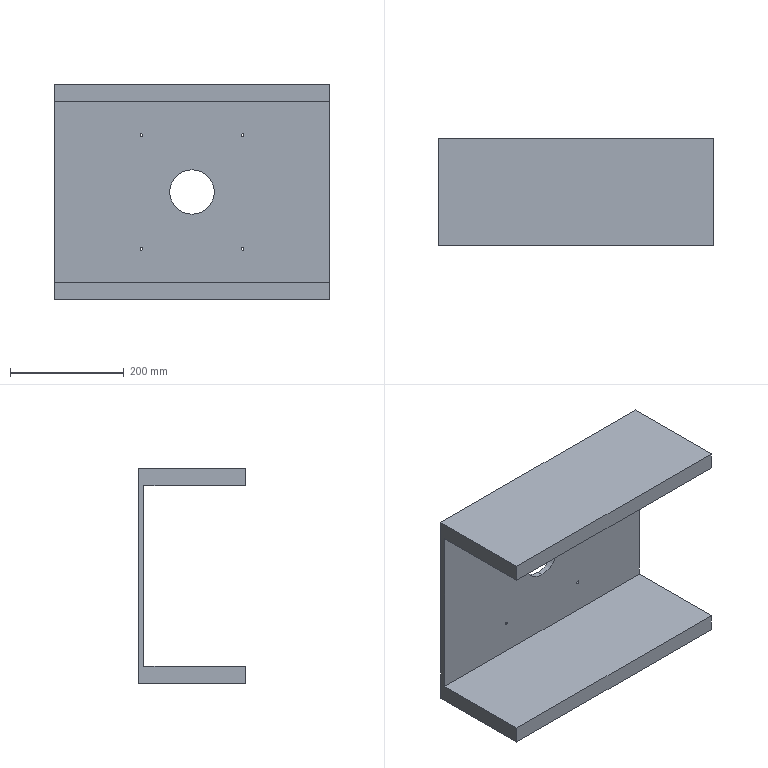Part | SolidWorks | features ICE 2, Extrusion 1 | 1 solid | 20 faces | box 484 x 189 x 378 mm | volume 6979121 mm3 | cylinder 10 | plane 10 | commonest cylinder face diameters 4.5 x8 78.113 x2
STEP:
#1=CARTESIAN_POINT('',(89.,179.,97.75));
#2=VERTEX_POINT('',#1);
#3=CARTESIAN_POINT('',(89.,179.,102.25));
#4=VERTEX_POINT('',#3);
#5=CARTESIAN_POINT('',(89.,179.,100.));
#6=DIRECTION('',(0.,1.,0.));
#7=DIRECTION('',(0.,0.,1.));
#8=AXIS2_PLACEMENT_3D('',#5,#6,#7);
#9=CIRCLE('',#8,2.25);
#10=EDGE_CURVE('',#2,#4,#9,.T.);
#11=ORIENTED_EDGE('',*,*,#10,.F.);
#12=CARTESIAN_POINT('',(89.,189.,97.75));
#13=VERTEX_POINT('',#12);
#14=CARTESIAN_POINT('',(89.,0.,97.75));
#15=DIRECTION('',(0.,1.,0.));
#16=VECTOR('',#15,1000.);
#17=LINE('',#14,#16);
#18=EDGE_CURVE('',#2,#13,#17,.T.);
#19=ORIENTED_EDGE('',*,*,#18,.T.);
#20=CARTESIAN_POINT('',(89.,189.,102.25));
#21=VERTEX_POINT('',#20);
#22=CARTESIAN_POINT('',(89.,189.,100.));
#23=DIRECTION('',(0.,1.,0.));
#24=DIRECTION('',(0.,0.,1.));
#25=AXIS2_PLACEMENT_3D('',#22,#23,#24);
#26=CIRCLE('',#25,2.25);
#27=EDGE_CURVE('',#13,#21,#26,.T.);
#28=ORIENTED_EDGE('',*,*,#27,.T.);
#29=CARTESIAN_POINT('',(89.,0.,102.25));
#30=DIRECTION('',(0.,1.,0.));
#31=VECTOR('',#30,1000.);
#32=LINE('',#29,#31);
#33=EDGE_CURVE('',#4,#21,#32,.T.);
#34=ORIENTED_EDGE('',*,*,#33,.F.);
#35=EDGE_LOOP('',(#11,#19,#28,#34));
#36=FACE_OUTER_BOUND('',#35,.T.);
#37=CARTESIAN_POINT('',(89.,0.,100.));
#38=DIRECTION('',(0.,1.,0.));
#39=DIRECTION('',(0.,0.,1.));
#40=AXIS2_PLACEMENT_3D('',#37,#38,#39);
#41=CYLINDRICAL_SURFACE('',#40,2.25);
#42=ADVANCED_FACE('',(#36),#41,.F.);
#43=CARTESIAN_POINT('',(-89.,179.,-102.25));
#44=VERTEX_POINT('',#43);
#45=CARTESIAN_POINT('',(-89.,179.,-97.75));
#46=VERTEX_POINT('',#45);
#47=CARTESIAN_POINT('',(-89.,179.,-100.));
#48=DIRECTION('',(0.,1.,0.));
#49=DIRECTION('',(0.,0.,1.));
#50=AXIS2_PLACEMENT_3D('',#47,#48,#49);
#51=CIRCLE('',#50,2.25);
#52=EDGE_CURVE('',#44,#46,#51,.T.);
#53=ORIENTED_EDGE('',*,*,#52,.F.);
#54=CARTESIAN_POINT('',(-89.,189.,-102.25));
#55=VERTEX_POINT('',#54);
#56=CARTESIAN_POINT('',(-89.,0.,-102.25));
#57=DIRECTION('',(0.,1.,0.));
#58=VECTOR('',#57,1000.);
#59=LINE('',#56,#58);
#60=EDGE_CURVE('',#44,#55,#59,.T.);
#61=ORIENTED_EDGE('',*,*,#60,.T.);
#62=CARTESIAN_POINT('',(-89.,189.,-97.75));
#63=VERTEX_POINT('',#62);
#64=CARTESIAN_POINT('',(-89.,189.,-100.));
#65=DIRECTION('',(0.,1.,0.));
#66=DIRECTION('',(0.,0.,1.));
#67=AXIS2_PLACEMENT_3D('',#64,#65,#66);
#68=CIRCLE('',#67,2.25);
#69=EDGE_CURVE('',#55,#63,#68,.T.);
#70=ORIENTED_EDGE('',*,*,#69,.T.);
#71=CARTESIAN_POINT('',(-89.,0.,-97.75));
#72=DIRECTION('',(0.,1.,0.));
#73=VECTOR('',#72,1000.);
#74=LINE('',#71,#73);
#75=EDGE_CURVE('',#46,#63,#74,.T.);
#76=ORIENTED_EDGE('',*,*,#75,.F.);
#77=EDGE_LOOP('',(#53,#61,#70,#76));
#78=FACE_OUTER_BOUND('',#77,.T.);
#79=CARTESIAN_POINT('',(-89.,0.,-100.));
#80=DIRECTION('',(0.,1.,0.));
#81=DIRECTION('',(0.,0.,1.));
#82=AXIS2_PLACEMENT_3D('',#79,#80,#81);
#83=CYLINDRICAL_SURFACE('',#82,2.25);
#84=ADVANCED_FACE('',(#78),#83,.F.);
#85=CARTESIAN_POINT('',(89.,179.,-102.25));
#86=VERTEX_POINT('',#85);
#87=CARTESIAN_POINT('',(89.,179.,-97.75));
#88=VERTEX_POINT('',#87);
#89=CARTESIAN_POINT('',(89.,179.,-100.));
#90=DIRECTION('',(0.,1.,0.));
#91=DIRECTION('',(0.,0.,1.));
#92=AXIS2_PLACEMENT_3D('',#89,#90,#91);
#93=CIRCLE('',#92,2.25);
#94=EDGE_CURVE('',#86,#88,#93,.T.);
#95=ORIENTED_EDGE('',*,*,#94,.F.);
#96=CARTESIAN_POINT('',(89.,189.,-102.25));
#97=VERTEX_POINT('',#96);
#98=CARTESIAN_POINT('',(89.,0.,-102.25));
#99=DIRECTION('',(0.,1.,0.));
#100=VECTOR('',#99,1000.);
#101=LINE('',#98,#100);
#102=EDGE_CURVE('',#86,#97,#101,.T.);
#103=ORIENTED_EDGE('',*,*,#102,.T.);
#104=CARTESIAN_POINT('',(89.,189.,-97.75));
#105=VERTEX_POINT('',#104);
#106=CARTESIAN_POINT('',(89.,189.,-100.));
#107=DIRECTION('',(0.,1.,0.));
#108=DIRECTION('',(0.,0.,1.));
#109=AXIS2_PLACEMENT_3D('',#106,#107,#108);
#110=CIRCLE('',#109,2.25);
#111=EDGE_CURVE('',#97,#105,#110,.T.);
#112=ORIENTED_EDGE('',*,*,#111,.T.);
#113=CARTESIAN_POINT('',(89.,0.,-97.75));
#114=DIRECTION('',(0.,1.,0.));
#115=VECTOR('',#114,1000.);
#116=LINE('',#113,#115);
#117=EDGE_CURVE('',#88,#105,#116,.T.);
#118=ORIENTED_EDGE('',*,*,#117,.F.);
#119=EDGE_LOOP('',(#95,#103,#112,#118));
#120=FACE_OUTER_BOUND('',#119,.T.);
#121=CARTESIAN_POINT('',(89.,0.,-100.));
#122=DIRECTION('',(0.,1.,0.));
#123=DIRECTION('',(0.,0.,1.));
#124=AXIS2_PLACEMENT_3D('',#121,#122,#123);
#125=CYLINDRICAL_SURFACE('',#124,2.25);
#126=ADVANCED_FACE('',(#120),#125,.F.);
#127=CARTESIAN_POINT('',(0.,179.,-39.057));
#128=VERTEX_POINT('',#127);
#129=CARTESIAN_POINT('',(0.,179.,39.057));
#130=VERTEX_POINT('',#129);
#131=CARTESIAN_POINT('',(0.,179.,0.));
#132=DIRECTION('',(0.,1.,0.));
#133=DIRECTION('',(0.,0.,1.));
#134=AXIS2_PLACEMENT_3D('',#131,#132,#133);
#135=CIRCLE('',#134,39.057);
#136=EDGE_CURVE('',#128,#130,#135,.T.);
#137=ORIENTED_EDGE('',*,*,#136,.F.);
#138=CARTESIAN_POINT('',(0.,189.,-39.057));
#139=VERTEX_POINT('',#138);
#140=CARTESIAN_POINT('',(0.,0.,-39.057));
#141=DIRECTION('',(0.,1.,0.));
#142=VECTOR('',#141,1000.);
#143=LINE('',#140,#142);
#144=EDGE_CURVE('',#128,#139,#143,.T.);
#145=ORIENTED_EDGE('',*,*,#144,.T.);
#146=CARTESIAN_POINT('',(0.,189.,39.057));
#147=VERTEX_POINT('',#146);
#148=CARTESIAN_POINT('',(0.,189.,0.));
#149=DIRECTION('',(0.,1.,0.));
#150=DIRECTION('',(0.,0.,1.));
#151=AXIS2_PLACEMENT_3D('',#148,#149,#150);
#152=CIRCLE('',#151,39.057);
#153=EDGE_CURVE('',#139,#147,#152,.T.);
#154=ORIENTED_EDGE('',*,*,#153,.T.);
#155=CARTESIAN_POINT('',(0.,0.,39.057));
#156=DIRECTION('',(0.,1.,0.));
#157=VECTOR('',#156,1000.);
#158=LINE('',#155,#157);
#159=EDGE_CURVE('',#130,#147,#158,.T.);
#160=ORIENTED_EDGE('',*,*,#159,.F.);
#161=EDGE_LOOP('',(#137,#145,#154,#160));
#162=FACE_OUTER_BOUND('',#161,.T.);
#163=CARTESIAN_POINT('',(0.,0.,0.));
#164=DIRECTION('',(0.,1.,0.));
#165=DIRECTION('',(0.,0.,1.));
#166=AXIS2_PLACEMENT_3D('',#163,#164,#165);
#167=CYLINDRICAL_SURFACE('',#166,39.057);
#168=ADVANCED_FACE('',(#162),#167,.F.);
#169=CARTESIAN_POINT('',(-89.,179.,97.75));
#170=VERTEX_POINT('',#169);
#171=CARTESIAN_POINT('',(-89.,179.,102.25));
#172=VERTEX_POINT('',#171);
#173=CARTESIAN_POINT('',(-89.,179.,100.));
#174=DIRECTION('',(0.,1.,0.));
#175=DIRECTION('',(0.,0.,1.));
#176=AXIS2_PLACEMENT_3D('',#173,#174,#175);
#177=CIRCLE('',#176,2.25);
#178=EDGE_CURVE('',#170,#172,#177,.T.);
#179=ORIENTED_EDGE('',*,*,#178,.F.);
#180=CARTESIAN_POINT('',(-89.,189.,97.75));
#181=VERTEX_POINT('',#180);
#182=CARTESIAN_POINT('',(-89.,0.,97.75));
#183=DIRECTION('',(0.,1.,0.));
#184=VECTOR('',#183,1000.);
#185=LINE('',#182,#184);
#186=EDGE_CURVE('',#170,#181,#185,.T.);
#187=ORIENTED_EDGE('',*,*,#186,.T.);
#188=CARTESIAN_POINT('',(-89.,189.,102.25));
#189=VERTEX_POINT('',#188);
#190=CARTESIAN_POINT('',(-89.,189.,100.));
#191=DIRECTION('',(0.,1.,0.));
#192=DIRECTION('',(0.,0.,1.));
#193=AXIS2_PLACEMENT_3D('',#190,#191,#192);
#194=CIRCLE('',#193,2.25);
#195=EDGE_CURVE('',#181,#189,#194,.T.);
#196=ORIENTED_EDGE('',*,*,#195,.T.);
#197=CARTESIAN_POINT('',(-89.,0.,102.25));
#198=DIRECTION('',(0.,1.,0.));
#199=VECTOR('',#198,1000.);
#200=LINE('',#197,#199);
#201=EDGE_CURVE('',#172,#189,#200,.T.);
#202=ORIENTED_EDGE('',*,*,#201,.F.);
#203=EDGE_LOOP('',(#179,#187,#196,#202));
#204=FACE_OUTER_BOUND('',#203,.T.);
#205=CARTESIAN_POINT('',(-89.,0.,100.));
#206=DIRECTION('',(0.,1.,0.));
#207=DIRECTION('',(0.,0.,1.));
#208=AXIS2_PLACEMENT_3D('',#205,#206,#207);
#209=CYLINDRICAL_SURFACE('',#208,2.25);
#210=ADVANCED_FACE('',(#204),#209,.F.);
#211=CARTESIAN_POINT('',(242.,0.,-159.));
#212=VERTEX_POINT('',#211);
#213=CARTESIAN_POINT('',(-242.,0.,-159.));
#214=VERTEX_POINT('',#213);
#215=CARTESIAN_POINT('',(242.,0.,-159.));
#216=DIRECTION('',(-1.,0.,0.));
#217=VECTOR('',#216,1000.);
#218=LINE('',#215,#217);
#219=EDGE_CURVE('',#212,#214,#218,.T.);
#220=ORIENTED_EDGE('',*,*,#219,.T.);
#221=CARTESIAN_POINT('',(-242.,0.,-189.));
#222=VERTEX_POINT('',#221);
#223=CARTESIAN_POINT('',(-242.,0.,189.));
#224=DIRECTION('',(0.,0.,1.));
#225=VECTOR('',#224,1000.);
#226=LINE('',#223,#225);
#227=EDGE_CURVE('',#222,#214,#226,.T.);
#228=ORIENTED_EDGE('',*,*,#227,.F.);
#229=CARTESIAN_POINT('',(242.,0.,-189.));
#230=VERTEX_POINT('',#229);
#231=CARTESIAN_POINT('',(-242.,0.,-189.));
#232=DIRECTION('',(-1.,0.,0.));
#233=VECTOR('',#232,1000.);
#234=LINE('',#231,#233);
#235=EDGE_CURVE('',#230,#222,#234,.T.);
#236=ORIENTED_EDGE('',*,*,#235,.F.);
#237=CARTESIAN_POINT('',(242.,0.,189.));
#238=DIRECTION('',(0.,0.,-1.));
#239=VECTOR('',#238,1000.);
#240=LINE('',#237,#239);
#241=EDGE_CURVE('',#212,#230,#240,.T.);
#242=ORIENTED_EDGE('',*,*,#241,.F.);
#243=EDGE_LOOP('',(#220,#228,#236,#242));
#244=FACE_OUTER_BOUND('',#243,.T.);
#245=CARTESIAN_POINT('',(0.,0.,0.));
#246=DIRECTION('',(0.,-1.,0.));
#247=DIRECTION('',(0.,0.,-1.));
#248=AXIS2_PLACEMENT_3D('',#245,#246,#247);
#249=PLANE('',#248);
#250=ADVANCED_FACE('',(#244),#249,.T.);
#251=CARTESIAN_POINT('',(242.,179.,159.));
#252=VERTEX_POINT('',#251);
#253=CARTESIAN_POINT('',(242.,179.,-159.));
#254=VERTEX_POINT('',#253);
#255=CARTESIAN_POINT('',(242.,179.,-159.));
#256=DIRECTION('',(0.,0.,-1.));
#257=VECTOR('',#256,1000.);
#258=LINE('',#255,#257);
#259=EDGE_CURVE('',#252,#254,#258,.T.);
#260=ORIENTED_EDGE('',*,*,#259,.T.);
#261=CARTESIAN_POINT('',(242.,0.,-159.));
#262=DIRECTION('',(0.,-1.,0.));
#263=VECTOR('',#262,1000.);
#264=LINE('',#261,#263);
#265=EDGE_CURVE('',#254,#212,#264,.T.);
#266=ORIENTED_EDGE('',*,*,#265,.T.);
#267=ORIENTED_EDGE('',*,*,#241,.T.);
#268=CARTESIAN_POINT('',(242.,189.,-189.));
#269=VERTEX_POINT('',#268);
#270=CARTESIAN_POINT('',(242.,189.,-189.));
#271=DIRECTION('',(0.,-1.,0.));
#272=VECTOR('',#271,1000.);
#273=LINE('',#270,#272);
#274=EDGE_CURVE('',#269,#230,#273,.T.);
#275=ORIENTED_EDGE('',*,*,#274,.F.);
#276=CARTESIAN_POINT('',(242.,189.,189.));
#277=VERTEX_POINT('',#276);
#278=CARTESIAN_POINT('',(242.,189.,189.));
#279=DIRECTION('',(0.,0.,-1.));
#280=VECTOR('',#279,1000.);
#281=LINE('',#278,#280);
#282=EDGE_CURVE('',#277,#269,#281,.T.);
#283=ORIENTED_EDGE('',*,*,#282,.F.);
#284=CARTESIAN_POINT('',(242.,0.,189.));
#285=VERTEX_POINT('',#284);
#286=CARTESIAN_POINT('',(242.,189.,189.));
#287=DIRECTION('',(0.,-1.,0.));
#288=VECTOR('',#287,1000.);
#289=LINE('',#286,#288);
#290=EDGE_CURVE('',#277,#285,#289,.T.);
#291=ORIENTED_EDGE('',*,*,#290,.T.);
#292=CARTESIAN_POINT('',(242.,0.,159.));
#293=VERTEX_POINT('',#292);
#294=CARTESIAN_POINT('',(242.,0.,189.));
#295=DIRECTION('',(0.,0.,-1.));
#296=VECTOR('',#295,1000.);
#297=LINE('',#294,#296);
#298=EDGE_CURVE('',#285,#293,#297,.T.);
#299=ORIENTED_EDGE('',*,*,#298,.T.);
#300=CARTESIAN_POINT('',(242.,0.,159.));
#301=DIRECTION('',(0.,1.,0.));
#302=VECTOR('',#301,1000.);
#303=LINE('',#300,#302);
#304=EDGE_CURVE('',#293,#252,#303,.T.);
#305=ORIENTED_EDGE('',*,*,#304,.T.);
#306=EDGE_LOOP('',(#260,#266,#267,#275,#283,#291,#299,#305));
#307=FACE_OUTER_BOUND('',#306,.T.);
#308=CARTESIAN_POINT('',(242.,189.,189.));
#309=DIRECTION('',(-1.,0.,0.));
#310=DIRECTION('',(0.,0.,1.));
#311=AXIS2_PLACEMENT_3D('',#308,#309,#310);
#312=PLANE('',#311);
#313=ADVANCED_FACE('',(#307),#312,.F.);
#314=ORIENTED_EDGE('',*,*,#235,.T.);
#315=CARTESIAN_POINT('',(-242.,189.,-189.));
#316=VERTEX_POINT('',#315);
#317=CARTESIAN_POINT('',(-242.,189.,-189.));
#318=DIRECTION('',(0.,-1.,0.));
#319=VECTOR('',#318,1000.);
#320=LINE('',#317,#319);
#321=EDGE_CURVE('',#316,#222,#320,.T.);
#322=ORIENTED_EDGE('',*,*,#321,.F.);
#323=CARTESIAN_POINT('',(-242.,189.,-189.));
#324=DIRECTION('',(-1.,0.,0.));
#325=VECTOR('',#324,1000.);
#326=LINE('',#323,#325);
#327=EDGE_CURVE('',#269,#316,#326,.T.);
#328=ORIENTED_EDGE('',*,*,#327,.F.);
#329=ORIENTED_EDGE('',*,*,#274,.T.);
#330=EDGE_LOOP('',(#314,#322,#328,#329));
#331=FACE_OUTER_BOUND('',#330,.T.);
#332=CARTESIAN_POINT('',(-242.,189.,-189.));
#333=DIRECTION('',(0.,0.,1.));
#334=DIRECTION('',(1.,0.,0.));
#335=AXIS2_PLACEMENT_3D('',#332,#333,#334);
#336=PLANE('',#335);
#337=ADVANCED_FACE('',(#331),#336,.F.);
#338=ORIENTED_EDGE('',*,*,#227,.T.);
#339=CARTESIAN_POINT('',(-242.,179.,-159.));
#340=VERTEX_POINT('',#339);
#341=CARTESIAN_POINT('',(-242.,0.,-159.));
#342=DIRECTION('',(0.,-1.,0.));
#343=VECTOR('',#342,1000.);
#344=LINE('',#341,#343);
#345=EDGE_CURVE('',#340,#214,#344,.T.);
#346=ORIENTED_EDGE('',*,*,#345,.F.);
#347=CARTESIAN_POINT('',(-242.,179.,159.));
#348=VERTEX_POINT('',#347);
#349=CARTESIAN_POINT('',(-242.,179.,-159.));
#350=DIRECTION('',(0.,0.,-1.));
#351=VECTOR('',#350,1000.);
#352=LINE('',#349,#351);
#353=EDGE_CURVE('',#348,#340,#352,.T.);
#354=ORIENTED_EDGE('',*,*,#353,.F.);
#355=CARTESIAN_POINT('',(-242.,0.,159.));
#356=VERTEX_POINT('',#355);
#357=CARTESIAN_POINT('',(-242.,0.,159.));
#358=DIRECTION('',(0.,1.,0.));
#359=VECTOR('',#358,1000.);
#360=LINE('',#357,#359);
#361=EDGE_CURVE('',#356,#348,#360,.T.);
#362=ORIENTED_EDGE('',*,*,#361,.F.);
#363=CARTESIAN_POINT('',(-242.,0.,189.));
#364=VERTEX_POINT('',#363);
#365=CARTESIAN_POINT('',(-242.,0.,189.));
#366=DIRECTION('',(0.,0.,1.));
#367=VECTOR('',#366,1000.);
#368=LINE('',#365,#367);
#369=EDGE_CURVE('',#356,#364,#368,.T.);
#370=ORIENTED_EDGE('',*,*,#369,.T.);
#371=CARTESIAN_POINT('',(-242.,189.,189.));
#372=VERTEX_POINT('',#371);
#373=CARTESIAN_POINT('',(-242.,189.,189.));
#374=DIRECTION('',(0.,-1.,0.));
#375=VECTOR('',#374,1000.);
#376=LINE('',#373,#375);
#377=EDGE_CURVE('',#372,#364,#376,.T.);
#378=ORIENTED_EDGE('',*,*,#377,.F.);
#379=CARTESIAN_POINT('',(-242.,189.,189.));
#380=DIRECTION('',(0.,0.,1.));
#381=VECTOR('',#380,1000.);
#382=LINE('',#379,#381);
#383=EDGE_CURVE('',#316,#372,#382,.T.);
#384=ORIENTED_EDGE('',*,*,#383,.F.);
#385=ORIENTED_EDGE('',*,*,#321,.T.);
#386=EDGE_LOOP('',(#338,#346,#354,#362,#370,#378,#384,#385));
#387=FACE_OUTER_BOUND('',#386,.T.);
#388=CARTESIAN_POINT('',(-242.,189.,189.));
#389=DIRECTION('',(1.,0.,0.));
#390=DIRECTION('',(0.,0.,-1.));
#391=AXIS2_PLACEMENT_3D('',#388,#389,#390);
#392=PLANE('',#391);
#393=ADVANCED_FACE('',(#387),#392,.F.);
#394=CARTESIAN_POINT('',(-242.,0.,189.));
#395=DIRECTION('',(1.,0.,0.));
#396=VECTOR('',#395,1000.);
#397=LINE('',#394,#396);
#398=EDGE_CURVE('',#364,#285,#397,.T.);
#399=ORIENTED_EDGE('',*,*,#398,.T.);
#400=ORIENTED_EDGE('',*,*,#290,.F.);
#401=CARTESIAN_POINT('',(-242.,189.,189.));
#402=DIRECTION('',(1.,0.,0.));
#403=VECTOR('',#402,1000.);
#404=LINE('',#401,#403);
#405=EDGE_CURVE('',#372,#277,#404,.T.);
#406=ORIENTED_EDGE('',*,*,#405,.F.);
#407=ORIENTED_EDGE('',*,*,#377,.T.);
#408=EDGE_LOOP('',(#399,#400,#406,#407));
#409=FACE_OUTER_BOUND('',#408,.T.);
#410=CARTESIAN_POINT('',(-242.,189.,189.));
#411=DIRECTION('',(0.,0.,-1.));
#412=DIRECTION('',(-1.,0.,0.));
#413=AXIS2_PLACEMENT_3D('',#410,#411,#412);
#414=PLANE('',#413);
#415=ADVANCED_FACE('',(#409),#414,.F.);
#416=CARTESIAN_POINT('',(89.,189.,100.));
#417=DIRECTION('',(0.,1.,0.));
#418=DIRECTION('',(0.,0.,1.));
#419=AXIS2_PLACEMENT_3D('',#416,#417,#418);
#420=CIRCLE('',#419,2.25);
#421=EDGE_CURVE('',#21,#13,#420,.T.);
#422=ORIENTED_EDGE('',*,*,#421,.F.);
#423=ORIENTED_EDGE('',*,*,#27,.F.);
#424=EDGE_LOOP('',(#422,#423));
#425=FACE_BOUND('',#424,.T.);
#426=CARTESIAN_POINT('',(-89.,189.,-100.));
#427=DIRECTION('',(0.,1.,0.));
#428=DIRECTION('',(0.,0.,1.));
#429=AXIS2_PLACEMENT_3D('',#426,#427,#428);
#430=CIRCLE('',#429,2.25);
#431=EDGE_CURVE('',#63,#55,#430,.T.);
#432=ORIENTED_EDGE('',*,*,#431,.F.);
#433=ORIENTED_EDGE('',*,*,#69,.F.);
#434=EDGE_LOOP('',(#432,#433));
#435=FACE_BOUND('',#434,.T.);
#436=CARTESIAN_POINT('',(89.,189.,-100.));
#437=DIRECTION('',(0.,1.,0.));
#438=DIRECTION('',(0.,0.,1.));
#439=AXIS2_PLACEMENT_3D('',#436,#437,#438);
#440=CIRCLE('',#439,2.25);
#441=EDGE_CURVE('',#105,#97,#440,.T.);
#442=ORIENTED_EDGE('',*,*,#441,.F.);
#443=ORIENTED_EDGE('',*,*,#111,.F.);
#444=EDGE_LOOP('',(#442,#443));
#445=FACE_BOUND('',#444,.T.);
#446=CARTESIAN_POINT('',(0.,189.,0.));
#447=DIRECTION('',(0.,1.,0.));
#448=DIRECTION('',(0.,0.,1.));
#449=AXIS2_PLACEMENT_3D('',#446,#447,#448);
#450=CIRCLE('',#449,39.057);
#451=EDGE_CURVE('',#147,#139,#450,.T.);
#452=ORIENTED_EDGE('',*,*,#451,.F.);
#453=ORIENTED_EDGE('',*,*,#153,.F.);
#454=EDGE_LOOP('',(#452,#453));
#455=FACE_BOUND('',#454,.T.);
#456=CARTESIAN_POINT('',(-89.,189.,100.));
#457=DIRECTION('',(0.,1.,0.));
#458=DIRECTION('',(0.,0.,1.));
#459=AXIS2_PLACEMENT_3D('',#456,#457,#458);
#460=CIRCLE('',#459,2.25);
#461=EDGE_CURVE('',#189,#181,#460,.T.);
#462=ORIENTED_EDGE('',*,*,#461,.F.);
#463=ORIENTED_EDGE('',*,*,#195,.F.);
#464=EDGE_LOOP('',(#462,#463));
#465=FACE_BOUND('',#464,.T.);
#466=ORIENTED_EDGE('',*,*,#282,.T.);
#467=ORIENTED_EDGE('',*,*,#327,.T.);
#468=ORIENTED_EDGE('',*,*,#383,.T.);
#469=ORIENTED_EDGE('',*,*,#405,.T.);
#470=EDGE_LOOP('',(#466,#467,#468,#469));
#471=FACE_OUTER_BOUND('',#470,.T.);
#472=CARTESIAN_POINT('',(0.,189.,0.));
#473=DIRECTION('',(0.,-1.,0.));
#474=DIRECTION('',(0.,0.,-1.));
#475=AXIS2_PLACEMENT_3D('',#472,#473,#474);
#476=PLANE('',#475);
#477=ADVANCED_FACE('',(#425,#435,#445,#455,#465,#471),#476,.F.);
#478=CARTESIAN_POINT('',(242.,0.,159.));
#479=DIRECTION('',(-1.,0.,0.));
#480=VECTOR('',#479,1000.);
#481=LINE('',#478,#480);
#482=EDGE_CURVE('',#293,#356,#481,.T.);
#483=ORIENTED_EDGE('',*,*,#482,.F.);
#484=ORIENTED_EDGE('',*,*,#298,.F.);
#485=ORIENTED_EDGE('',*,*,#398,.F.);
#486=ORIENTED_EDGE('',*,*,#369,.F.);
#487=EDGE_LOOP('',(#483,#484,#485,#486));
#488=FACE_OUTER_BOUND('',#487,.T.);
#489=CARTESIAN_POINT('',(0.,0.,0.));
#490=DIRECTION('',(0.,-1.,0.));
#491=DIRECTION('',(0.,0.,-1.));
#492=AXIS2_PLACEMENT_3D('',#489,#490,#491);
#493=PLANE('',#492);
#494=ADVANCED_FACE('',(#488),#493,.T.);
#495=ORIENTED_EDGE('',*,*,#345,.T.);
#496=ORIENTED_EDGE('',*,*,#219,.F.);
#497=ORIENTED_EDGE('',*,*,#265,.F.);
#498=CARTESIAN_POINT('',(242.,179.,-159.));
#499=DIRECTION('',(-1.,0.,0.));
#500=VECTOR('',#499,1000.);
#501=LINE('',#498,#500);
#502=EDGE_CURVE('',#254,#340,#501,.T.);
#503=ORIENTED_EDGE('',*,*,#502,.T.);
#504=EDGE_LOOP('',(#495,#496,#497,#503));
#505=FACE_OUTER_BOUND('',#504,.T.);
#506=CARTESIAN_POINT('',(242.,0.,-159.));
#507=DIRECTION('',(0.,0.,-1.));
#508=DIRECTION('',(-1.,0.,0.));
#509=AXIS2_PLACEMENT_3D('',#506,#507,#508);
#510=PLANE('',#509);
#511=ADVANCED_FACE('',(#505),#510,.F.);
#512=CARTESIAN_POINT('',(89.,179.,100.));
#513=DIRECTION('',(0.,1.,0.));
#514=DIRECTION('',(0.,0.,1.));
#515=AXIS2_PLACEMENT_3D('',#512,#513,#514);
#516=CIRCLE('',#515,2.25);
#517=EDGE_CURVE('',#4,#2,#516,.T.);
#518=ORIENTED_EDGE('',*,*,#517,.T.);
#519=ORIENTED_EDGE('',*,*,#10,.T.);
#520=EDGE_LOOP('',(#518,#519));
#521=FACE_BOUND('',#520,.T.);
#522=CARTESIAN_POINT('',(-89.,179.,-100.));
#523=DIRECTION('',(0.,1.,0.));
#524=DIRECTION('',(0.,0.,1.));
#525=AXIS2_PLACEMENT_3D('',#522,#523,#524);
#526=CIRCLE('',#525,2.25);
#527=EDGE_CURVE('',#46,#44,#526,.T.);
#528=ORIENTED_EDGE('',*,*,#527,.T.);
#529=ORIENTED_EDGE('',*,*,#52,.T.);
#530=EDGE_LOOP('',(#528,#529));
#531=FACE_BOUND('',#530,.T.);
#532=CARTESIAN_POINT('',(89.,179.,-100.));
#533=DIRECTION('',(0.,1.,0.));
#534=DIRECTION('',(0.,0.,1.));
#535=AXIS2_PLACEMENT_3D('',#532,#533,#534);
#536=CIRCLE('',#535,2.25);
#537=EDGE_CURVE('',#88,#86,#536,.T.);
#538=ORIENTED_EDGE('',*,*,#537,.T.);
#539=ORIENTED_EDGE('',*,*,#94,.T.);
#540=EDGE_LOOP('',(#538,#539));
#541=FACE_BOUND('',#540,.T.);
#542=CARTESIAN_POINT('',(0.,179.,0.));
#543=DIRECTION('',(0.,1.,0.));
#544=DIRECTION('',(0.,0.,1.));
#545=AXIS2_PLACEMENT_3D('',#542,#543,#544);
#546=CIRCLE('',#545,39.057);
#547=EDGE_CURVE('',#130,#128,#546,.T.);
#548=ORIENTED_EDGE('',*,*,#547,.T.);
#549=ORIENTED_EDGE('',*,*,#136,.T.);
#550=EDGE_LOOP('',(#548,#549));
#551=FACE_BOUND('',#550,.T.);
#552=CARTESIAN_POINT('',(-89.,179.,100.));
#553=DIRECTION('',(0.,1.,0.));
#554=DIRECTION('',(0.,0.,1.));
#555=AXIS2_PLACEMENT_3D('',#552,#553,#554);
#556=CIRCLE('',#555,2.25);
#557=EDGE_CURVE('',#172,#170,#556,.T.);
#558=ORIENTED_EDGE('',*,*,#557,.T.);
#559=ORIENTED_EDGE('',*,*,#178,.T.);
#560=EDGE_LOOP('',(#558,#559));
#561=FACE_BOUND('',#560,.T.);
#562=ORIENTED_EDGE('',*,*,#353,.T.);
#563=ORIENTED_EDGE('',*,*,#502,.F.);
#564=ORIENTED_EDGE('',*,*,#259,.F.);
#565=CARTESIAN_POINT('',(242.,179.,159.));
#566=DIRECTION('',(-1.,0.,0.));
#567=VECTOR('',#566,1000.);
#568=LINE('',#565,#567);
#569=EDGE_CURVE('',#252,#348,#568,.T.);
#570=ORIENTED_EDGE('',*,*,#569,.T.);
#571=EDGE_LOOP('',(#562,#563,#564,#570));
#572=FACE_OUTER_BOUND('',#571,.T.);
#573=CARTESIAN_POINT('',(242.,179.,-159.));
#574=DIRECTION('',(0.,1.,0.));
#575=DIRECTION('',(0.,0.,1.));
#576=AXIS2_PLACEMENT_3D('',#573,#574,#575);
#577=PLANE('',#576);
#578=ADVANCED_FACE('',(#521,#531,#541,#551,#561,#572),#577,.F.);
#579=ORIENTED_EDGE('',*,*,#361,.T.);
#580=ORIENTED_EDGE('',*,*,#569,.F.);
#581=ORIENTED_EDGE('',*,*,#304,.F.);
#582=ORIENTED_EDGE('',*,*,#482,.T.);
#583=EDGE_LOOP('',(#579,#580,#581,#582));
#584=FACE_OUTER_BOUND('',#583,.T.);
#585=CARTESIAN_POINT('',(242.,0.,159.));
#586=DIRECTION('',(0.,0.,1.));
#587=DIRECTION('',(1.,0.,0.));
#588=AXIS2_PLACEMENT_3D('',#585,#586,#587);
#589=PLANE('',#588);
#590=ADVANCED_FACE('',(#584),#589,.F.);
#591=ORIENTED_EDGE('',*,*,#186,.F.);
#592=ORIENTED_EDGE('',*,*,#557,.F.);
#593=ORIENTED_EDGE('',*,*,#201,.T.);
#594=ORIENTED_EDGE('',*,*,#461,.T.);
#595=EDGE_LOOP('',(#591,#592,#593,#594));
#596=FACE_OUTER_BOUND('',#595,.T.);
#597=CARTESIAN_POINT('',(-89.,0.,100.));
#598=DIRECTION('',(0.,1.,0.));
#599=DIRECTION('',(0.,0.,1.));
#600=AXIS2_PLACEMENT_3D('',#597,#598,#599);
#601=CYLINDRICAL_SURFACE('',#600,2.25);
#602=ADVANCED_FACE('',(#596),#601,.F.);
#603=ORIENTED_EDGE('',*,*,#144,.F.);
#604=ORIENTED_EDGE('',*,*,#547,.F.);
#605=ORIENTED_EDGE('',*,*,#159,.T.);
#606=ORIENTED_EDGE('',*,*,#451,.T.);
#607=EDGE_LOOP('',(#603,#604,#605,#606));
#608=FACE_OUTER_BOUND('',#607,.T.);
#609=CARTESIAN_POINT('',(0.,0.,0.));
#610=DIRECTION('',(0.,1.,0.));
#611=DIRECTION('',(0.,0.,1.));
#612=AXIS2_PLACEMENT_3D('',#609,#610,#611);
#613=CYLINDRICAL_SURFACE('',#612,39.057);
#614=ADVANCED_FACE('',(#608),#613,.F.);
#615=ORIENTED_EDGE('',*,*,#102,.F.);
#616=ORIENTED_EDGE('',*,*,#537,.F.);
#617=ORIENTED_EDGE('',*,*,#117,.T.);
#618=ORIENTED_EDGE('',*,*,#441,.T.);
#619=EDGE_LOOP('',(#615,#616,#617,#618));
#620=FACE_OUTER_BOUND('',#619,.T.);
#621=CARTESIAN_POINT('',(89.,0.,-100.));
#622=DIRECTION('',(0.,1.,0.));
#623=DIRECTION('',(0.,0.,1.));
#624=AXIS2_PLACEMENT_3D('',#621,#622,#623);
#625=CYLINDRICAL_SURFACE('',#624,2.25);
#626=ADVANCED_FACE('',(#620),#625,.F.);
#627=ORIENTED_EDGE('',*,*,#60,.F.);
#628=ORIENTED_EDGE('',*,*,#527,.F.);
#629=ORIENTED_EDGE('',*,*,#75,.T.);
#630=ORIENTED_EDGE('',*,*,#431,.T.);
#631=EDGE_LOOP('',(#627,#628,#629,#630));
#632=FACE_OUTER_BOUND('',#631,.T.);
#633=CARTESIAN_POINT('',(-89.,0.,-100.));
#634=DIRECTION('',(0.,1.,0.));
#635=DIRECTION('',(0.,0.,1.));
#636=AXIS2_PLACEMENT_3D('',#633,#634,#635);
#637=CYLINDRICAL_SURFACE('',#636,2.25);
#638=ADVANCED_FACE('',(#632),#637,.F.);
#639=ORIENTED_EDGE('',*,*,#18,.F.);
#640=ORIENTED_EDGE('',*,*,#517,.F.);
#641=ORIENTED_EDGE('',*,*,#33,.T.);
#642=ORIENTED_EDGE('',*,*,#421,.T.);
#643=EDGE_LOOP('',(#639,#640,#641,#642));
#644=FACE_OUTER_BOUND('',#643,.T.);
#645=CARTESIAN_POINT('',(89.,0.,100.));
#646=DIRECTION('',(0.,1.,0.));
#647=DIRECTION('',(0.,0.,1.));
#648=AXIS2_PLACEMENT_3D('',#645,#646,#647);
#649=CYLINDRICAL_SURFACE('',#648,2.25);
#650=ADVANCED_FACE('',(#644),#649,.F.);
#651=CLOSED_SHELL('',(#42,#84,#126,#168,#210,#250,#313,#337,#393,#415,#477,#494,#511,#578,#590,#602,#614,#626,#638,#650));
#652=MANIFOLD_SOLID_BREP('',#651);
#653=CARTESIAN_POINT('',(0.,0.,0.));
#654=DIRECTION('',(0.,0.,1.));
#655=DIRECTION('',(1.,0.,0.));
#656=AXIS2_PLACEMENT_3D('',#653,#654,#655);
#657=(LENGTH_UNIT()NAMED_UNIT(*)SI_UNIT(.MILLI.,.METRE.));
#658=UNCERTAINTY_MEASURE_WITH_UNIT(LENGTH_MEASURE(0.00001),#657,'','');
#659=(NAMED_UNIT(*)PLANE_ANGLE_UNIT()SI_UNIT($,.RADIAN.));
#660=(NAMED_UNIT(*)SI_UNIT($,.STERADIAN.)SOLID_ANGLE_UNIT());
#661=(GEOMETRIC_REPRESENTATION_CONTEXT(3)GLOBAL_UNCERTAINTY_ASSIGNED_CONTEXT((#658))GLOBAL_UNIT_ASSIGNED_CONTEXT((#657,#659,#660))REPRESENTATION_CONTEXT('',''));
#662=ADVANCED_BREP_SHAPE_REPRESENTATION('',(#652,#656),#661);